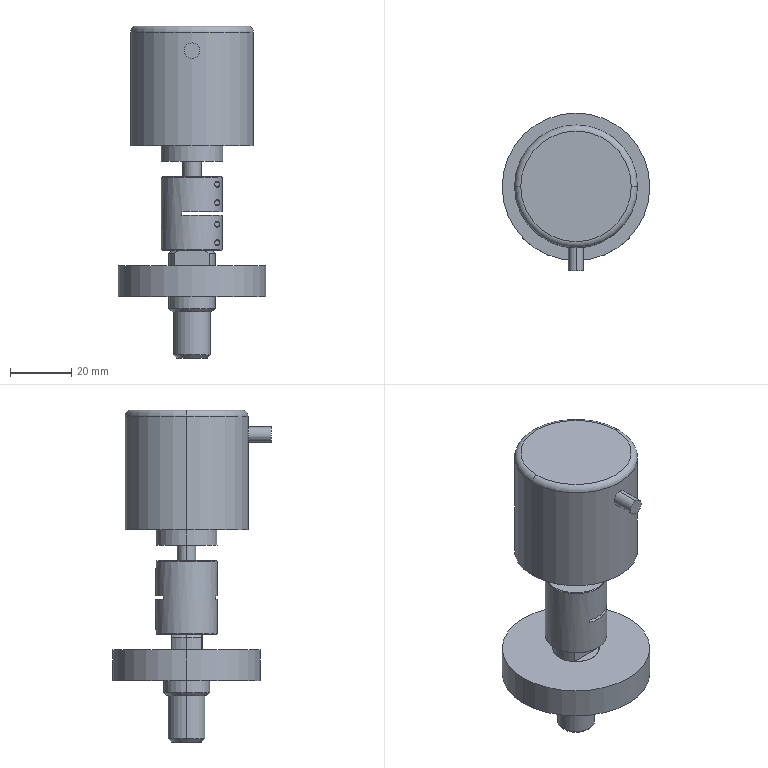Part | SolidWorks | features CompositeCurve 3 | 6 solids | 162 faces | box 48 x 51.5 x 108 mm | volume 78961 mm3 | plane 69 | cylinder 65 | cone 26 | torus 2 | commonest cylinder face diameters 2 x18 2.286 x8 2.667 x8 20 x7 2.5 x6 6 x6